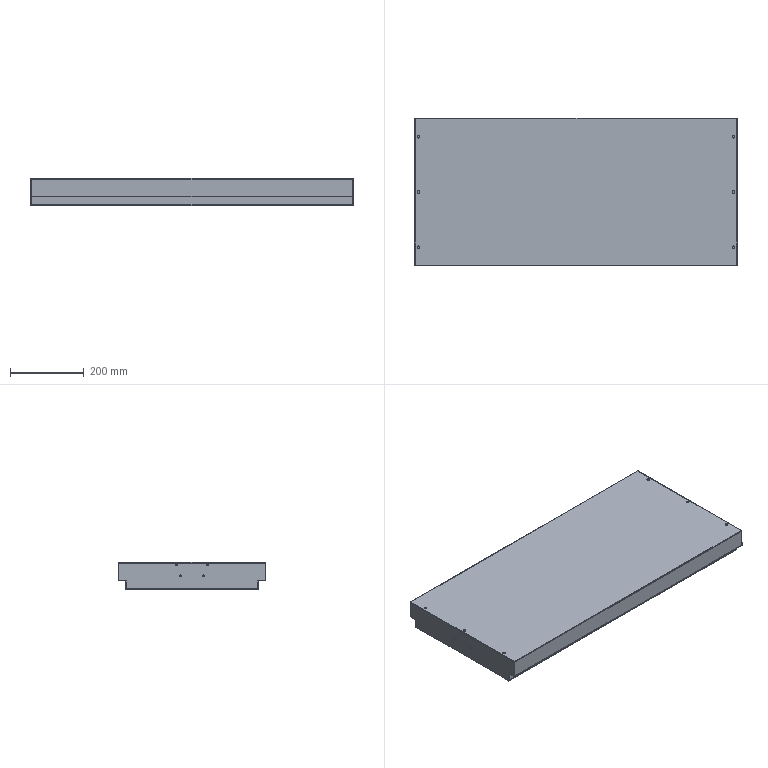Part | SolidWorks | features EdgeFlange 5, ICE 2, SMBaseFlange 2, CornerFeat 1, Cut 1, FlatPattern 1, SheetMetal 1 | 1 solid | 150 faces | box 875 x 400 x 73.5 mm | volume 926748 mm3 | plane 98 | cylinder 44 | spline 8 | commonest cylinder face diameters 0.4 x12 3.4 x12 7 x12 5 x8